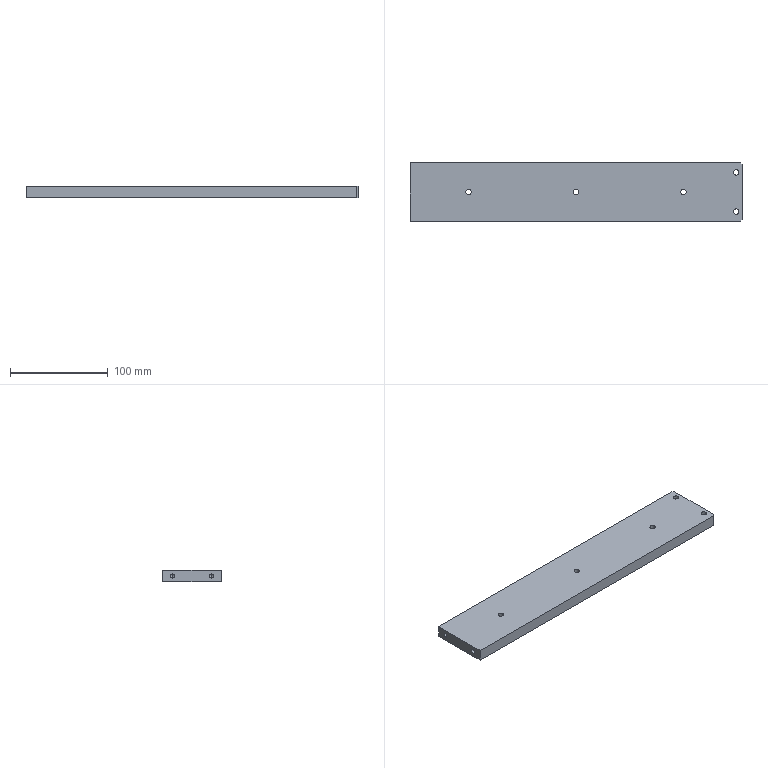Part | SolidWorks | features HoleWzd 3, Chamfer 1, Extrusion 1 | 1 solid | 41 faces | box 340 x 60 x 12 mm | volume 241410 mm3 | cylinder 24 | plane 13 | cone 4 | commonest cylinder face diameters 5.5 x10 10 x10 4.2 x4
STEP:
#1=CARTESIAN_POINT('',(115.,0.,-0.3));
#2=VERTEX_POINT('',#1);
#3=CARTESIAN_POINT('',(105.,0.,-0.3));
#4=VERTEX_POINT('',#3);
#5=CARTESIAN_POINT('',(110.,0.,-0.3));
#6=DIRECTION('',(0.,0.,-1.));
#7=DIRECTION('',(-1.,0.,0.));
#8=AXIS2_PLACEMENT_3D('',#5,#6,#7);
#9=CIRCLE('',#8,5.);
#10=EDGE_CURVE('',#2,#4,#9,.T.);
#11=ORIENTED_EDGE('',*,*,#10,.F.);
#12=CARTESIAN_POINT('',(115.,0.,-6.));
#13=VERTEX_POINT('',#12);
#14=CARTESIAN_POINT('',(115.,0.,-6.));
#15=DIRECTION('',(0.,0.,-1.));
#16=VECTOR('',#15,1000.);
#17=LINE('',#14,#16);
#18=EDGE_CURVE('',#2,#13,#17,.T.);
#19=ORIENTED_EDGE('',*,*,#18,.T.);
#20=CARTESIAN_POINT('',(105.,0.,-6.));
#21=VERTEX_POINT('',#20);
#22=CARTESIAN_POINT('',(110.,0.,-6.));
#23=DIRECTION('',(0.,0.,-1.));
#24=DIRECTION('',(-1.,0.,0.));
#25=AXIS2_PLACEMENT_3D('',#22,#23,#24);
#26=CIRCLE('',#25,5.);
#27=EDGE_CURVE('',#13,#21,#26,.T.);
#28=ORIENTED_EDGE('',*,*,#27,.T.);
#29=CARTESIAN_POINT('',(105.,0.,-6.));
#30=DIRECTION('',(0.,0.,-1.));
#31=VECTOR('',#30,1000.);
#32=LINE('',#29,#31);
#33=EDGE_CURVE('',#4,#21,#32,.T.);
#34=ORIENTED_EDGE('',*,*,#33,.F.);
#35=EDGE_LOOP('',(#11,#19,#28,#34));
#36=FACE_OUTER_BOUND('',#35,.T.);
#37=CARTESIAN_POINT('',(110.,0.,-6.));
#38=DIRECTION('',(0.,0.,-1.));
#39=DIRECTION('',(-1.,0.,0.));
#40=AXIS2_PLACEMENT_3D('',#37,#38,#39);
#41=CYLINDRICAL_SURFACE('',#40,5.);
#42=ADVANCED_FACE('',(#36),#41,.F.);
#43=CARTESIAN_POINT('',(112.75,0.,6.));
#44=VERTEX_POINT('',#43);
#45=CARTESIAN_POINT('',(107.25,0.,6.));
#46=VERTEX_POINT('',#45);
#47=CARTESIAN_POINT('',(110.,0.,6.));
#48=DIRECTION('',(0.,0.,-1.));
#49=DIRECTION('',(-1.,0.,0.));
#50=AXIS2_PLACEMENT_3D('',#47,#48,#49);
#51=CIRCLE('',#50,2.75);
#52=EDGE_CURVE('',#44,#46,#51,.T.);
#53=ORIENTED_EDGE('',*,*,#52,.F.);
#54=CARTESIAN_POINT('',(112.75,0.,-0.3));
#55=VERTEX_POINT('',#54);
#56=CARTESIAN_POINT('',(112.75,0.,-6.));
#57=DIRECTION('',(0.,0.,-1.));
#58=VECTOR('',#57,1000.);
#59=LINE('',#56,#58);
#60=EDGE_CURVE('',#44,#55,#59,.T.);
#61=ORIENTED_EDGE('',*,*,#60,.T.);
#62=CARTESIAN_POINT('',(107.25,0.,-0.3));
#63=VERTEX_POINT('',#62);
#64=CARTESIAN_POINT('',(110.,0.,-0.3));
#65=DIRECTION('',(0.,0.,-1.));
#66=DIRECTION('',(-1.,0.,0.));
#67=AXIS2_PLACEMENT_3D('',#64,#65,#66);
#68=CIRCLE('',#67,2.75);
#69=EDGE_CURVE('',#55,#63,#68,.T.);
#70=ORIENTED_EDGE('',*,*,#69,.T.);
#71=CARTESIAN_POINT('',(107.25,0.,-6.));
#72=DIRECTION('',(0.,0.,-1.));
#73=VECTOR('',#72,1000.);
#74=LINE('',#71,#73);
#75=EDGE_CURVE('',#46,#63,#74,.T.);
#76=ORIENTED_EDGE('',*,*,#75,.F.);
#77=EDGE_LOOP('',(#53,#61,#70,#76));
#78=FACE_OUTER_BOUND('',#77,.T.);
#79=CARTESIAN_POINT('',(110.,0.,-6.));
#80=DIRECTION('',(0.,0.,-1.));
#81=DIRECTION('',(-1.,0.,0.));
#82=AXIS2_PLACEMENT_3D('',#79,#80,#81);
#83=CYLINDRICAL_SURFACE('',#82,2.75);
#84=ADVANCED_FACE('',(#78),#83,.F.);
#85=CARTESIAN_POINT('',(-105.,0.,-0.3));
#86=VERTEX_POINT('',#85);
#87=CARTESIAN_POINT('',(-115.,0.,-0.3));
#88=VERTEX_POINT('',#87);
#89=CARTESIAN_POINT('',(-110.,0.,-0.3));
#90=DIRECTION('',(0.,0.,-1.));
#91=DIRECTION('',(-1.,0.,0.));
#92=AXIS2_PLACEMENT_3D('',#89,#90,#91);
#93=CIRCLE('',#92,5.);
#94=EDGE_CURVE('',#86,#88,#93,.T.);
#95=ORIENTED_EDGE('',*,*,#94,.F.);
#96=CARTESIAN_POINT('',(-105.,0.,-6.));
#97=VERTEX_POINT('',#96);
#98=CARTESIAN_POINT('',(-105.,0.,-6.));
#99=DIRECTION('',(0.,0.,-1.));
#100=VECTOR('',#99,1000.);
#101=LINE('',#98,#100);
#102=EDGE_CURVE('',#86,#97,#101,.T.);
#103=ORIENTED_EDGE('',*,*,#102,.T.);
#104=CARTESIAN_POINT('',(-115.,0.,-6.));
#105=VERTEX_POINT('',#104);
#106=CARTESIAN_POINT('',(-110.,0.,-6.));
#107=DIRECTION('',(0.,0.,-1.));
#108=DIRECTION('',(-1.,0.,0.));
#109=AXIS2_PLACEMENT_3D('',#106,#107,#108);
#110=CIRCLE('',#109,5.);
#111=EDGE_CURVE('',#97,#105,#110,.T.);
#112=ORIENTED_EDGE('',*,*,#111,.T.);
#113=CARTESIAN_POINT('',(-115.,0.,-6.));
#114=DIRECTION('',(0.,0.,-1.));
#115=VECTOR('',#114,1000.);
#116=LINE('',#113,#115);
#117=EDGE_CURVE('',#88,#105,#116,.T.);
#118=ORIENTED_EDGE('',*,*,#117,.F.);
#119=EDGE_LOOP('',(#95,#103,#112,#118));
#120=FACE_OUTER_BOUND('',#119,.T.);
#121=CARTESIAN_POINT('',(-110.,0.,-6.));
#122=DIRECTION('',(0.,0.,-1.));
#123=DIRECTION('',(-1.,0.,0.));
#124=AXIS2_PLACEMENT_3D('',#121,#122,#123);
#125=CYLINDRICAL_SURFACE('',#124,5.);
#126=ADVANCED_FACE('',(#120),#125,.F.);
#127=CARTESIAN_POINT('',(-107.25,0.,6.));
#128=VERTEX_POINT('',#127);
#129=CARTESIAN_POINT('',(-112.75,0.,6.));
#130=VERTEX_POINT('',#129);
#131=CARTESIAN_POINT('',(-110.,0.,6.));
#132=DIRECTION('',(0.,0.,-1.));
#133=DIRECTION('',(-1.,0.,0.));
#134=AXIS2_PLACEMENT_3D('',#131,#132,#133);
#135=CIRCLE('',#134,2.75);
#136=EDGE_CURVE('',#128,#130,#135,.T.);
#137=ORIENTED_EDGE('',*,*,#136,.F.);
#138=CARTESIAN_POINT('',(-107.25,0.,-0.3));
#139=VERTEX_POINT('',#138);
#140=CARTESIAN_POINT('',(-107.25,0.,-6.));
#141=DIRECTION('',(0.,0.,-1.));
#142=VECTOR('',#141,1000.);
#143=LINE('',#140,#142);
#144=EDGE_CURVE('',#128,#139,#143,.T.);
#145=ORIENTED_EDGE('',*,*,#144,.T.);
#146=CARTESIAN_POINT('',(-112.75,0.,-0.3));
#147=VERTEX_POINT('',#146);
#148=CARTESIAN_POINT('',(-110.,0.,-0.3));
#149=DIRECTION('',(0.,0.,-1.));
#150=DIRECTION('',(-1.,0.,0.));
#151=AXIS2_PLACEMENT_3D('',#148,#149,#150);
#152=CIRCLE('',#151,2.75);
#153=EDGE_CURVE('',#139,#147,#152,.T.);
#154=ORIENTED_EDGE('',*,*,#153,.T.);
#155=CARTESIAN_POINT('',(-112.75,0.,-6.));
#156=DIRECTION('',(0.,0.,-1.));
#157=VECTOR('',#156,1000.);
#158=LINE('',#155,#157);
#159=EDGE_CURVE('',#130,#147,#158,.T.);
#160=ORIENTED_EDGE('',*,*,#159,.F.);
#161=EDGE_LOOP('',(#137,#145,#154,#160));
#162=FACE_OUTER_BOUND('',#161,.T.);
#163=CARTESIAN_POINT('',(-110.,0.,-6.));
#164=DIRECTION('',(0.,0.,-1.));
#165=DIRECTION('',(-1.,0.,0.));
#166=AXIS2_PLACEMENT_3D('',#163,#164,#165);
#167=CYLINDRICAL_SURFACE('',#166,2.75);
#168=ADVANCED_FACE('',(#162),#167,.F.);
#169=CARTESIAN_POINT('',(5.,0.,-0.3));
#170=VERTEX_POINT('',#169);
#171=CARTESIAN_POINT('',(-5.,0.,-0.3));
#172=VERTEX_POINT('',#171);
#173=CARTESIAN_POINT('',(0.,0.,-0.3));
#174=DIRECTION('',(0.,0.,-1.));
#175=DIRECTION('',(-1.,0.,0.));
#176=AXIS2_PLACEMENT_3D('',#173,#174,#175);
#177=CIRCLE('',#176,5.);
#178=EDGE_CURVE('',#170,#172,#177,.T.);
#179=ORIENTED_EDGE('',*,*,#178,.F.);
#180=CARTESIAN_POINT('',(5.,0.,-6.));
#181=VERTEX_POINT('',#180);
#182=CARTESIAN_POINT('',(5.,0.,-6.));
#183=DIRECTION('',(0.,0.,-1.));
#184=VECTOR('',#183,1000.);
#185=LINE('',#182,#184);
#186=EDGE_CURVE('',#170,#181,#185,.T.);
#187=ORIENTED_EDGE('',*,*,#186,.T.);
#188=CARTESIAN_POINT('',(-5.,0.,-6.));
#189=VERTEX_POINT('',#188);
#190=CARTESIAN_POINT('',(0.,0.,-6.));
#191=DIRECTION('',(0.,0.,-1.));
#192=DIRECTION('',(-1.,0.,0.));
#193=AXIS2_PLACEMENT_3D('',#190,#191,#192);
#194=CIRCLE('',#193,5.);
#195=EDGE_CURVE('',#181,#189,#194,.T.);
#196=ORIENTED_EDGE('',*,*,#195,.T.);
#197=CARTESIAN_POINT('',(-5.,0.,-6.));
#198=DIRECTION('',(0.,0.,-1.));
#199=VECTOR('',#198,1000.);
#200=LINE('',#197,#199);
#201=EDGE_CURVE('',#172,#189,#200,.T.);
#202=ORIENTED_EDGE('',*,*,#201,.F.);
#203=EDGE_LOOP('',(#179,#187,#196,#202));
#204=FACE_OUTER_BOUND('',#203,.T.);
#205=CARTESIAN_POINT('',(0.,0.,-6.));
#206=DIRECTION('',(0.,0.,-1.));
#207=DIRECTION('',(-1.,0.,0.));
#208=AXIS2_PLACEMENT_3D('',#205,#206,#207);
#209=CYLINDRICAL_SURFACE('',#208,5.);
#210=ADVANCED_FACE('',(#204),#209,.F.);
#211=CARTESIAN_POINT('',(2.75,0.,6.));
#212=VERTEX_POINT('',#211);
#213=CARTESIAN_POINT('',(-2.75,0.,6.));
#214=VERTEX_POINT('',#213);
#215=CARTESIAN_POINT('',(0.,0.,6.));
#216=DIRECTION('',(0.,0.,-1.));
#217=DIRECTION('',(-1.,0.,0.));
#218=AXIS2_PLACEMENT_3D('',#215,#216,#217);
#219=CIRCLE('',#218,2.75);
#220=EDGE_CURVE('',#212,#214,#219,.T.);
#221=ORIENTED_EDGE('',*,*,#220,.F.);
#222=CARTESIAN_POINT('',(2.75,0.,-0.3));
#223=VERTEX_POINT('',#222);
#224=CARTESIAN_POINT('',(2.75,0.,-6.));
#225=DIRECTION('',(0.,0.,-1.));
#226=VECTOR('',#225,1000.);
#227=LINE('',#224,#226);
#228=EDGE_CURVE('',#212,#223,#227,.T.);
#229=ORIENTED_EDGE('',*,*,#228,.T.);
#230=CARTESIAN_POINT('',(-2.75,0.,-0.3));
#231=VERTEX_POINT('',#230);
#232=CARTESIAN_POINT('',(0.,0.,-0.3));
#233=DIRECTION('',(0.,0.,-1.));
#234=DIRECTION('',(-1.,0.,0.));
#235=AXIS2_PLACEMENT_3D('',#232,#233,#234);
#236=CIRCLE('',#235,2.75);
#237=EDGE_CURVE('',#223,#231,#236,.T.);
#238=ORIENTED_EDGE('',*,*,#237,.T.);
#239=CARTESIAN_POINT('',(-2.75,0.,-6.));
#240=DIRECTION('',(0.,0.,-1.));
#241=VECTOR('',#240,1000.);
#242=LINE('',#239,#241);
#243=EDGE_CURVE('',#214,#231,#242,.T.);
#244=ORIENTED_EDGE('',*,*,#243,.F.);
#245=EDGE_LOOP('',(#221,#229,#238,#244));
#246=FACE_OUTER_BOUND('',#245,.T.);
#247=CARTESIAN_POINT('',(0.,0.,-6.));
#248=DIRECTION('',(0.,0.,-1.));
#249=DIRECTION('',(-1.,0.,0.));
#250=AXIS2_PLACEMENT_3D('',#247,#248,#249);
#251=CYLINDRICAL_SURFACE('',#250,2.75);
#252=ADVANCED_FACE('',(#246),#251,.F.);
#253=CARTESIAN_POINT('',(169.,20.,-0.3));
#254=VERTEX_POINT('',#253);
#255=CARTESIAN_POINT('',(159.,20.,-0.3));
#256=VERTEX_POINT('',#255);
#257=CARTESIAN_POINT('',(164.,20.,-0.3));
#258=DIRECTION('',(0.,0.,-1.));
#259=DIRECTION('',(-1.,0.,0.));
#260=AXIS2_PLACEMENT_3D('',#257,#258,#259);
#261=CIRCLE('',#260,5.);
#262=EDGE_CURVE('',#254,#256,#261,.T.);
#263=ORIENTED_EDGE('',*,*,#262,.F.);
#264=CARTESIAN_POINT('',(169.,20.,-6.));
#265=VERTEX_POINT('',#264);
#266=CARTESIAN_POINT('',(169.,20.,-6.));
#267=DIRECTION('',(0.,0.,-1.));
#268=VECTOR('',#267,1000.);
#269=LINE('',#266,#268);
#270=EDGE_CURVE('',#254,#265,#269,.T.);
#271=ORIENTED_EDGE('',*,*,#270,.T.);
#272=CARTESIAN_POINT('',(159.,20.,-6.));
#273=VERTEX_POINT('',#272);
#274=CARTESIAN_POINT('',(164.,20.,-6.));
#275=DIRECTION('',(0.,0.,-1.));
#276=DIRECTION('',(-1.,0.,0.));
#277=AXIS2_PLACEMENT_3D('',#274,#275,#276);
#278=CIRCLE('',#277,5.);
#279=EDGE_CURVE('',#265,#273,#278,.T.);
#280=ORIENTED_EDGE('',*,*,#279,.T.);
#281=CARTESIAN_POINT('',(159.,20.,-6.));
#282=DIRECTION('',(0.,0.,-1.));
#283=VECTOR('',#282,1000.);
#284=LINE('',#281,#283);
#285=EDGE_CURVE('',#256,#273,#284,.T.);
#286=ORIENTED_EDGE('',*,*,#285,.F.);
#287=EDGE_LOOP('',(#263,#271,#280,#286));
#288=FACE_OUTER_BOUND('',#287,.T.);
#289=CARTESIAN_POINT('',(164.,20.,-6.));
#290=DIRECTION('',(0.,0.,-1.));
#291=DIRECTION('',(-1.,0.,0.));
#292=AXIS2_PLACEMENT_3D('',#289,#290,#291);
#293=CYLINDRICAL_SURFACE('',#292,5.);
#294=ADVANCED_FACE('',(#288),#293,.F.);
#295=CARTESIAN_POINT('',(166.75,20.,6.));
#296=VERTEX_POINT('',#295);
#297=CARTESIAN_POINT('',(161.25,20.,6.));
#298=VERTEX_POINT('',#297);
#299=CARTESIAN_POINT('',(164.,20.,6.));
#300=DIRECTION('',(0.,0.,-1.));
#301=DIRECTION('',(-1.,0.,0.));
#302=AXIS2_PLACEMENT_3D('',#299,#300,#301);
#303=CIRCLE('',#302,2.75);
#304=EDGE_CURVE('',#296,#298,#303,.T.);
#305=ORIENTED_EDGE('',*,*,#304,.F.);
#306=CARTESIAN_POINT('',(166.75,20.,-0.3));
#307=VERTEX_POINT('',#306);
#308=CARTESIAN_POINT('',(166.75,20.,-6.));
#309=DIRECTION('',(0.,0.,-1.));
#310=VECTOR('',#309,1000.);
#311=LINE('',#308,#310);
#312=EDGE_CURVE('',#296,#307,#311,.T.);
#313=ORIENTED_EDGE('',*,*,#312,.T.);
#314=CARTESIAN_POINT('',(161.25,20.,-0.3));
#315=VERTEX_POINT('',#314);
#316=CARTESIAN_POINT('',(164.,20.,-0.3));
#317=DIRECTION('',(0.,0.,-1.));
#318=DIRECTION('',(-1.,0.,0.));
#319=AXIS2_PLACEMENT_3D('',#316,#317,#318);
#320=CIRCLE('',#319,2.75);
#321=EDGE_CURVE('',#307,#315,#320,.T.);
#322=ORIENTED_EDGE('',*,*,#321,.T.);
#323=CARTESIAN_POINT('',(161.25,20.,-6.));
#324=DIRECTION('',(0.,0.,-1.));
#325=VECTOR('',#324,1000.);
#326=LINE('',#323,#325);
#327=EDGE_CURVE('',#298,#315,#326,.T.);
#328=ORIENTED_EDGE('',*,*,#327,.F.);
#329=EDGE_LOOP('',(#305,#313,#322,#328));
#330=FACE_OUTER_BOUND('',#329,.T.);
#331=CARTESIAN_POINT('',(164.,20.,-6.));
#332=DIRECTION('',(0.,0.,-1.));
#333=DIRECTION('',(-1.,0.,0.));
#334=AXIS2_PLACEMENT_3D('',#331,#332,#333);
#335=CYLINDRICAL_SURFACE('',#334,2.75);
#336=ADVANCED_FACE('',(#330),#335,.F.);
#337=CARTESIAN_POINT('',(169.,-20.,-0.3));
#338=VERTEX_POINT('',#337);
#339=CARTESIAN_POINT('',(159.,-20.,-0.3));
#340=VERTEX_POINT('',#339);
#341=CARTESIAN_POINT('',(164.,-20.,-0.3));
#342=DIRECTION('',(0.,0.,-1.));
#343=DIRECTION('',(-1.,0.,0.));
#344=AXIS2_PLACEMENT_3D('',#341,#342,#343);
#345=CIRCLE('',#344,5.);
#346=EDGE_CURVE('',#338,#340,#345,.T.);
#347=ORIENTED_EDGE('',*,*,#346,.F.);
#348=CARTESIAN_POINT('',(169.,-20.,-6.));
#349=VERTEX_POINT('',#348);
#350=CARTESIAN_POINT('',(169.,-20.,-6.));
#351=DIRECTION('',(0.,0.,-1.));
#352=VECTOR('',#351,1000.);
#353=LINE('',#350,#352);
#354=EDGE_CURVE('',#338,#349,#353,.T.);
#355=ORIENTED_EDGE('',*,*,#354,.T.);
#356=CARTESIAN_POINT('',(159.,-20.,-6.));
#357=VERTEX_POINT('',#356);
#358=CARTESIAN_POINT('',(164.,-20.,-6.));
#359=DIRECTION('',(0.,0.,-1.));
#360=DIRECTION('',(-1.,0.,0.));
#361=AXIS2_PLACEMENT_3D('',#358,#359,#360);
#362=CIRCLE('',#361,5.);
#363=EDGE_CURVE('',#349,#357,#362,.T.);
#364=ORIENTED_EDGE('',*,*,#363,.T.);
#365=CARTESIAN_POINT('',(159.,-20.,-6.));
#366=DIRECTION('',(0.,0.,-1.));
#367=VECTOR('',#366,1000.);
#368=LINE('',#365,#367);
#369=EDGE_CURVE('',#340,#357,#368,.T.);
#370=ORIENTED_EDGE('',*,*,#369,.F.);
#371=EDGE_LOOP('',(#347,#355,#364,#370));
#372=FACE_OUTER_BOUND('',#371,.T.);
#373=CARTESIAN_POINT('',(164.,-20.,-6.));
#374=DIRECTION('',(0.,0.,-1.));
#375=DIRECTION('',(-1.,0.,0.));
#376=AXIS2_PLACEMENT_3D('',#373,#374,#375);
#377=CYLINDRICAL_SURFACE('',#376,5.);
#378=ADVANCED_FACE('',(#372),#377,.F.);
#379=CARTESIAN_POINT('',(166.75,-20.,6.));
#380=VERTEX_POINT('',#379);
#381=CARTESIAN_POINT('',(161.25,-20.,6.));
#382=VERTEX_POINT('',#381);
#383=CARTESIAN_POINT('',(164.,-20.,6.));
#384=DIRECTION('',(0.,0.,-1.));
#385=DIRECTION('',(-1.,0.,0.));
#386=AXIS2_PLACEMENT_3D('',#383,#384,#385);
#387=CIRCLE('',#386,2.75);
#388=EDGE_CURVE('',#380,#382,#387,.T.);
#389=ORIENTED_EDGE('',*,*,#388,.F.);
#390=CARTESIAN_POINT('',(166.75,-20.,-0.3));
#391=VERTEX_POINT('',#390);
#392=CARTESIAN_POINT('',(166.75,-20.,-6.));
#393=DIRECTION('',(0.,0.,-1.));
#394=VECTOR('',#393,1000.);
#395=LINE('',#392,#394);
#396=EDGE_CURVE('',#380,#391,#395,.T.);
#397=ORIENTED_EDGE('',*,*,#396,.T.);
#398=CARTESIAN_POINT('',(161.25,-20.,-0.3));
#399=VERTEX_POINT('',#398);
#400=CARTESIAN_POINT('',(164.,-20.,-0.3));
#401=DIRECTION('',(0.,0.,-1.));
#402=DIRECTION('',(-1.,0.,0.));
#403=AXIS2_PLACEMENT_3D('',#400,#401,#402);
#404=CIRCLE('',#403,2.75);
#405=EDGE_CURVE('',#391,#399,#404,.T.);
#406=ORIENTED_EDGE('',*,*,#405,.T.);
#407=CARTESIAN_POINT('',(161.25,-20.,-6.));
#408=DIRECTION('',(0.,0.,-1.));
#409=VECTOR('',#408,1000.);
#410=LINE('',#407,#409);
#411=EDGE_CURVE('',#382,#399,#410,.T.);
#412=ORIENTED_EDGE('',*,*,#411,.F.);
#413=EDGE_LOOP('',(#389,#397,#406,#412));
#414=FACE_OUTER_BOUND('',#413,.T.);
#415=CARTESIAN_POINT('',(164.,-20.,-6.));
#416=DIRECTION('',(0.,0.,-1.));
#417=DIRECTION('',(-1.,0.,0.));
#418=AXIS2_PLACEMENT_3D('',#415,#416,#417);
#419=CYLINDRICAL_SURFACE('',#418,2.75);
#420=ADVANCED_FACE('',(#414),#419,.F.);
#421=CARTESIAN_POINT('',(-157.6,20.,-2.1));
#422=VERTEX_POINT('',#421);
#423=CARTESIAN_POINT('',(-157.6,20.,2.1));
#424=VERTEX_POINT('',#423);
#425=CARTESIAN_POINT('',(-157.6,20.,0.));
#426=DIRECTION('',(-1.,0.,0.));
#427=DIRECTION('',(0.,0.,1.));
#428=AXIS2_PLACEMENT_3D('',#425,#426,#427);
#429=CIRCLE('',#428,2.1);
#430=EDGE_CURVE('',#422,#424,#429,.T.);
#431=ORIENTED_EDGE('',*,*,#430,.F.);
#432=CARTESIAN_POINT('',(-170.,20.,-2.1));
#433=VERTEX_POINT('',#432);
#434=CARTESIAN_POINT('',(-170.,20.,-2.1));
#435=DIRECTION('',(-1.,0.,0.));
#436=VECTOR('',#435,1000.);
#437=LINE('',#434,#436);
#438=EDGE_CURVE('',#422,#433,#437,.T.);
#439=ORIENTED_EDGE('',*,*,#438,.T.);
#440=CARTESIAN_POINT('',(-170.,20.,2.1));
#441=VERTEX_POINT('',#440);
#442=CARTESIAN_POINT('',(-170.,20.,0.));
#443=DIRECTION('',(-1.,0.,0.));
#444=DIRECTION('',(0.,0.,1.));
#445=AXIS2_PLACEMENT_3D('',#442,#443,#444);
#446=CIRCLE('',#445,2.1);
#447=EDGE_CURVE('',#433,#441,#446,.T.);
#448=ORIENTED_EDGE('',*,*,#447,.T.);
#449=CARTESIAN_POINT('',(-170.,20.,2.1));
#450=DIRECTION('',(-1.,0.,0.));
#451=VECTOR('',#450,1000.);
#452=LINE('',#449,#451);
#453=EDGE_CURVE('',#424,#441,#452,.T.);
#454=ORIENTED_EDGE('',*,*,#453,.F.);
#455=EDGE_LOOP('',(#431,#439,#448,#454));
#456=FACE_OUTER_BOUND('',#455,.T.);
#457=CARTESIAN_POINT('',(-170.,20.,0.));
#458=DIRECTION('',(-1.,0.,0.));
#459=DIRECTION('',(0.,0.,1.));
#460=AXIS2_PLACEMENT_3D('',#457,#458,#459);
#461=CYLINDRICAL_SURFACE('',#460,2.1);
#462=ADVANCED_FACE('',(#456),#461,.F.);
#463=CARTESIAN_POINT('',(-156.338,20.,0.));
#464=VERTEX_POINT('',#463);
#465=CARTESIAN_POINT('',(-157.6,20.,2.1));
#466=DIRECTION('',(-0.515,0.,0.8572));
#467=VECTOR('',#466,1000.);
#468=LINE('',#465,#467);
#469=EDGE_CURVE('',#464,#424,#468,.T.);
#470=ORIENTED_EDGE('',*,*,#469,.F.);
#471=CARTESIAN_POINT('',(-157.6,20.,-2.1));
#472=DIRECTION('',(-0.515,0.,-0.8572));
#473=VECTOR('',#472,1000.);
#474=LINE('',#471,#473);
#475=EDGE_CURVE('',#464,#422,#474,.T.);
#476=ORIENTED_EDGE('',*,*,#475,.T.);
#477=ORIENTED_EDGE('',*,*,#430,.T.);
#478=EDGE_LOOP('',(#470,#476,#477));
#479=FACE_OUTER_BOUND('',#478,.T.);
#480=CARTESIAN_POINT('',(-157.6,20.,0.));
#481=DIRECTION('',(-1.,0.,0.));
#482=DIRECTION('',(0.,0.,1.));
#483=AXIS2_PLACEMENT_3D('',#480,#481,#482);
#484=CONICAL_SURFACE('',#483,2.1,1.03);
#485=ADVANCED_FACE('',(#479),#484,.F.);
#486=CARTESIAN_POINT('',(-157.6,-20.,-2.1));
#487=VERTEX_POINT('',#486);
#488=CARTESIAN_POINT('',(-157.6,-20.,2.1));
#489=VERTEX_POINT('',#488);
#490=CARTESIAN_POINT('',(-157.6,-20.,0.));
#491=DIRECTION('',(-1.,0.,0.));
#492=DIRECTION('',(0.,0.,1.));
#493=AXIS2_PLACEMENT_3D('',#490,#491,#492);
#494=CIRCLE('',#493,2.1);
#495=EDGE_CURVE('',#487,#489,#494,.T.);
#496=ORIENTED_EDGE('',*,*,#495,.F.);
#497=CARTESIAN_POINT('',(-170.,-20.,-2.1));
#498=VERTEX_POINT('',#497);
#499=CARTESIAN_POINT('',(-170.,-20.,-2.1));
#500=DIRECTION('',(-1.,0.,0.));
#501=VECTOR('',#500,1000.);
#502=LINE('',#499,#501);
#503=EDGE_CURVE('',#487,#498,#502,.T.);
#504=ORIENTED_EDGE('',*,*,#503,.T.);
#505=CARTESIAN_POINT('',(-170.,-20.,2.1));
#506=VERTEX_POINT('',#505);
#507=CARTESIAN_POINT('',(-170.,-20.,0.));
#508=DIRECTION('',(-1.,0.,0.));
#509=DIRECTION('',(0.,0.,1.));
#510=AXIS2_PLACEMENT_3D('',#507,#508,#509);
#511=CIRCLE('',#510,2.1);
#512=EDGE_CURVE('',#498,#506,#511,.T.);
#513=ORIENTED_EDGE('',*,*,#512,.T.);
#514=CARTESIAN_POINT('',(-170.,-20.,2.1));
#515=DIRECTION('',(-1.,0.,0.));
#516=VECTOR('',#515,1000.);
#517=LINE('',#514,#516);
#518=EDGE_CURVE('',#489,#506,#517,.T.);
#519=ORIENTED_EDGE('',*,*,#518,.F.);
#520=EDGE_LOOP('',(#496,#504,#513,#519));
#521=FACE_OUTER_BOUND('',#520,.T.);
#522=CARTESIAN_POINT('',(-170.,-20.,0.));
#523=DIRECTION('',(-1.,0.,0.));
#524=DIRECTION('',(0.,0.,1.));
#525=AXIS2_PLACEMENT_3D('',#522,#523,#524);
#526=CYLINDRICAL_SURFACE('',#525,2.1);
#527=ADVANCED_FACE('',(#521),#526,.F.);
#528=CARTESIAN_POINT('',(-156.338,-20.,0.));
#529=VERTEX_POINT('',#528);
#530=CARTESIAN_POINT('',(-157.6,-20.,2.1));
#531=DIRECTION('',(-0.515,0.,0.8572));
#532=VECTOR('',#531,1000.);
#533=LINE('',#530,#532);
#534=EDGE_CURVE('',#529,#489,#533,.T.);
#535=ORIENTED_EDGE('',*,*,#534,.F.);
#536=CARTESIAN_POINT('',(-157.6,-20.,-2.1));
#537=DIRECTION('',(-0.515,0.,-0.8572));
#538=VECTOR('',#537,1000.);
#539=LINE('',#536,#538);
#540=EDGE_CURVE('',#529,#487,#539,.T.);
#541=ORIENTED_EDGE('',*,*,#540,.T.);
#542=ORIENTED_EDGE('',*,*,#495,.T.);
#543=EDGE_LOOP('',(#535,#541,#542));
#544=FACE_OUTER_BOUND('',#543,.T.);
#545=CARTESIAN_POINT('',(-157.6,-20.,0.));
#546=DIRECTION('',(-1.,0.,0.));
#547=DIRECTION('',(0.,0.,1.));
#548=AXIS2_PLACEMENT_3D('',#545,#546,#547);
#549=CONICAL_SURFACE('',#548,2.1,1.03);
#550=ADVANCED_FACE('',(#544),#549,.F.);
#551=CARTESIAN_POINT('',(170.,-28.,6.));
#552=VERTEX_POINT('',#551);
#553=CARTESIAN_POINT('',(170.,28.,6.));
#554=VERTEX_POINT('',#553);
#555=CARTESIAN_POINT('',(170.,-30.,6.));
#556=DIRECTION('',(0.,1.,0.));
#557=VECTOR('',#556,1000.);
#558=LINE('',#555,#557);
#559=EDGE_CURVE('',#552,#554,#558,.T.);
#560=ORIENTED_EDGE('',*,*,#559,.F.);
#561=CARTESIAN_POINT('',(170.,-28.,-6.));
#562=VERTEX_POINT('',#561);
#563=CARTESIAN_POINT('',(170.,-28.,6.));
#564=DIRECTION('',(0.,0.,-1.));
#565=VECTOR('',#564,1000.);
#566=LINE('',#563,#565);
#567=EDGE_CURVE('',#552,#562,#566,.T.);
#568=ORIENTED_EDGE('',*,*,#567,.T.);
#569=CARTESIAN_POINT('',(170.,28.,-6.));
#570=VERTEX_POINT('',#569);
#571=CARTESIAN_POINT('',(170.,-30.,-6.));
#572=DIRECTION('',(0.,1.,0.));
#573=VECTOR('',#572,1000.);
#574=LINE('',#571,#573);
#575=EDGE_CURVE('',#562,#570,#574,.T.);
#576=ORIENTED_EDGE('',*,*,#575,.T.);
#577=CARTESIAN_POINT('',(170.,28.,6.));
#578=DIRECTION('',(0.,0.,1.));
#579=VECTOR('',#578,1000.);
#580=LINE('',#577,#579);
#581=EDGE_CURVE('',#570,#554,#580,.T.);
#582=ORIENTED_EDGE('',*,*,#581,.T.);
#583=EDGE_LOOP('',(#560,#568,#576,#582));
#584=FACE_OUTER_BOUND('',#583,.T.);
#585=CARTESIAN_POINT('',(170.,-30.,6.));
#586=DIRECTION('',(-1.,0.,0.));
#587=DIRECTION('',(0.,0.,1.));
#588=AXIS2_PLACEMENT_3D('',#585,#586,#587);
#589=PLANE('',#588);
#590=ADVANCED_FACE('',(#584),#589,.F.);
#591=CARTESIAN_POINT('',(168.,30.,6.));
#592=VERTEX_POINT('',#591);
#593=CARTESIAN_POINT('',(-170.,30.,6.));
#594=VERTEX_POINT('',#593);
#595=CARTESIAN_POINT('',(-170.,30.,6.));
#596=DIRECTION('',(-1.,0.,0.));
#597=VECTOR('',#596,1000.);
#598=LINE('',#595,#597);
#599=EDGE_CURVE('',#592,#594,#598,.T.);
#600=ORIENTED_EDGE('',*,*,#599,.F.);
#601=CARTESIAN_POINT('',(168.,30.,-6.));
#602=VERTEX_POINT('',#601);
#603=CARTESIAN_POINT('',(168.,30.,6.));
#604=DIRECTION('',(0.,0.,-1.));
#605=VECTOR('',#604,1000.);
#606=LINE('',#603,#605);
#607=EDGE_CURVE('',#592,#602,#606,.T.);
#608=ORIENTED_EDGE('',*,*,#607,.T.);
#609=CARTESIAN_POINT('',(-170.,30.,-6.));
#610=VERTEX_POINT('',#609);
#611=CARTESIAN_POINT('',(-170.,30.,-6.));
#612=DIRECTION('',(-1.,0.,0.));
#613=VECTOR('',#612,1000.);
#614=LINE('',#611,#613);
#615=EDGE_CURVE('',#602,#610,#614,.T.);
#616=ORIENTED_EDGE('',*,*,#615,.T.);
#617=CARTESIAN_POINT('',(-170.,30.,6.));
#618=DIRECTION('',(0.,0.,-1.));
#619=VECTOR('',#618,1000.);
#620=LINE('',#617,#619);
#621=EDGE_CURVE('',#594,#610,#620,.T.);
#622=ORIENTED_EDGE('',*,*,#621,.F.);
#623=EDGE_LOOP('',(#600,#608,#616,#622));
#624=FACE_OUTER_BOUND('',#623,.T.);
#625=CARTESIAN_POINT('',(-170.,30.,6.));
#626=DIRECTION('',(0.,-1.,0.));
#627=DIRECTION('',(0.,0.,-1.));
#628=AXIS2_PLACEMENT_3D('',#625,#626,#627);
#629=PLANE('',#628);
#630=ADVANCED_FACE('',(#624),#629,.F.);
#631=CARTESIAN_POINT('',(-170.,20.,0.));
#632=DIRECTION('',(-1.,0.,0.));
#633=DIRECTION('',(0.,0.,1.));
#634=AXIS2_PLACEMENT_3D('',#631,#632,#633);
#635=CIRCLE('',#634,2.1);
#636=EDGE_CURVE('',#441,#433,#635,.T.);
#637=ORIENTED_EDGE('',*,*,#636,.F.);
#638=ORIENTED_EDGE('',*,*,#447,.F.);
#639=EDGE_LOOP('',(#637,#638));
#640=FACE_BOUND('',#639,.T.);
#641=CARTESIAN_POINT('',(-170.,-20.,0.));
#642=DIRECTION('',(-1.,0.,0.));
#643=DIRECTION('',(0.,0.,1.));
#644=AXIS2_PLACEMENT_3D('',#641,#642,#643);
#645=CIRCLE('',#644,2.1);
#646=EDGE_CURVE('',#506,#498,#645,.T.);
#647=ORIENTED_EDGE('',*,*,#646,.F.);
#648=ORIENTED_EDGE('',*,*,#512,.F.);
#649=EDGE_LOOP('',(#647,#648));
#650=FACE_BOUND('',#649,.T.);
#651=CARTESIAN_POINT('',(-170.,-30.,-6.));
#652=VERTEX_POINT('',#651);
#653=CARTESIAN_POINT('',(-170.,-30.,-6.));
#654=DIRECTION('',(0.,-1.,0.));
#655=VECTOR('',#654,1000.);
#656=LINE('',#653,#655);
#657=EDGE_CURVE('',#610,#652,#656,.T.);
#658=ORIENTED_EDGE('',*,*,#657,.T.);
#659=CARTESIAN_POINT('',(-170.,-30.,6.));
#660=VERTEX_POINT('',#659);
#661=CARTESIAN_POINT('',(-170.,-30.,6.));
#662=DIRECTION('',(0.,0.,-1.));
#663=VECTOR('',#662,1000.);
#664=LINE('',#661,#663);
#665=EDGE_CURVE('',#660,#652,#664,.T.);
#666=ORIENTED_EDGE('',*,*,#665,.F.);
#667=CARTESIAN_POINT('',(-170.,-30.,6.));
#668=DIRECTION('',(0.,-1.,0.));
#669=VECTOR('',#668,1000.);
#670=LINE('',#667,#669);
#671=EDGE_CURVE('',#594,#660,#670,.T.);
#672=ORIENTED_EDGE('',*,*,#671,.F.);
#673=ORIENTED_EDGE('',*,*,#621,.T.);
#674=EDGE_LOOP('',(#658,#666,#672,#673));
#675=FACE_OUTER_BOUND('',#674,.T.);
#676=CARTESIAN_POINT('',(-170.,-30.,6.));
#677=DIRECTION('',(1.,0.,0.));
#678=DIRECTION('',(0.,0.,-1.));
#679=AXIS2_PLACEMENT_3D('',#676,#677,#678);
#680=PLANE('',#679);
#681=ADVANCED_FACE('',(#640,#650,#675),#680,.F.);
#682=CARTESIAN_POINT('',(168.,-30.,-6.));
#683=VERTEX_POINT('',#682);
#684=CARTESIAN_POINT('',(-170.,-30.,-6.));
#685=DIRECTION('',(1.,0.,0.));
#686=VECTOR('',#685,1000.);
#687=LINE('',#684,#686);
#688=EDGE_CURVE('',#652,#683,#687,.T.);
#689=ORIENTED_EDGE('',*,*,#688,.T.);
#690=CARTESIAN_POINT('',(168.,-30.,6.));
#691=VERTEX_POINT('',#690);
#692=CARTESIAN_POINT('',(168.,-30.,6.));
#693=DIRECTION('',(0.,0.,1.));
#694=VECTOR('',#693,1000.);
#695=LINE('',#692,#694);
#696=EDGE_CURVE('',#683,#691,#695,.T.);
#697=ORIENTED_EDGE('',*,*,#696,.T.);
#698=CARTESIAN_POINT('',(-170.,-30.,6.));
#699=DIRECTION('',(1.,0.,0.));
#700=VECTOR('',#699,1000.);
#701=LINE('',#698,#700);
#702=EDGE_CURVE('',#660,#691,#701,.T.);
#703=ORIENTED_EDGE('',*,*,#702,.F.);
#704=ORIENTED_EDGE('',*,*,#665,.T.);
#705=EDGE_LOOP('',(#689,#697,#703,#704));
#706=FACE_OUTER_BOUND('',#705,.T.);
#707=CARTESIAN_POINT('',(-170.,-30.,6.));
#708=DIRECTION('',(0.,1.,0.));
#709=DIRECTION('',(0.,0.,1.));
#710=AXIS2_PLACEMENT_3D('',#707,#708,#709);
#711=PLANE('',#710);
#712=ADVANCED_FACE('',(#706),#711,.F.);
#713=CARTESIAN_POINT('',(110.,0.,6.));
#714=DIRECTION('',(0.,0.,-1.));
#715=DIRECTION('',(-1.,0.,0.));
#716=AXIS2_PLACEMENT_3D('',#713,#714,#715);
#717=CIRCLE('',#716,2.75);
#718=EDGE_CURVE('',#46,#44,#717,.T.);
#719=ORIENTED_EDGE('',*,*,#718,.T.);
#720=ORIENTED_EDGE('',*,*,#52,.T.);
#721=EDGE_LOOP('',(#719,#720));
#722=FACE_BOUND('',#721,.T.);
#723=CARTESIAN_POINT('',(-110.,0.,6.));
#724=DIRECTION('',(0.,0.,-1.));
#725=DIRECTION('',(-1.,0.,0.));
#726=AXIS2_PLACEMENT_3D('',#723,#724,#725);
#727=CIRCLE('',#726,2.75);
#728=EDGE_CURVE('',#130,#128,#727,.T.);
#729=ORIENTED_EDGE('',*,*,#728,.T.);
#730=ORIENTED_EDGE('',*,*,#136,.T.);
#731=EDGE_LOOP('',(#729,#730));
#732=FACE_BOUND('',#731,.T.);
#733=CARTESIAN_POINT('',(0.,0.,6.));
#734=DIRECTION('',(0.,0.,-1.));
#735=DIRECTION('',(-1.,0.,0.));
#736=AXIS2_PLACEMENT_3D('',#733,#734,#735);
#737=CIRCLE('',#736,2.75);
#738=EDGE_CURVE('',#214,#212,#737,.T.);
#739=ORIENTED_EDGE('',*,*,#738,.T.);
#740=ORIENTED_EDGE('',*,*,#220,.T.);
#741=EDGE_LOOP('',(#739,#740));
#742=FACE_BOUND('',#741,.T.);
#743=CARTESIAN_POINT('',(164.,20.,6.));
#744=DIRECTION('',(0.,0.,-1.));
#745=DIRECTION('',(-1.,0.,0.));
#746=AXIS2_PLACEMENT_3D('',#743,#744,#745);
#747=CIRCLE('',#746,2.75);
#748=EDGE_CURVE('',#298,#296,#747,.T.);
#749=ORIENTED_EDGE('',*,*,#748,.T.);
#750=ORIENTED_EDGE('',*,*,#304,.T.);
#751=EDGE_LOOP('',(#749,#750));
#752=FACE_BOUND('',#751,.T.);
#753=CARTESIAN_POINT('',(164.,-20.,6.));
#754=DIRECTION('',(0.,0.,-1.));
#755=DIRECTION('',(-1.,0.,0.));
#756=AXIS2_PLACEMENT_3D('',#753,#754,#755);
#757=CIRCLE('',#756,2.75);
#758=EDGE_CURVE('',#382,#380,#757,.T.);
#759=ORIENTED_EDGE('',*,*,#758,.T.);
#760=ORIENTED_EDGE('',*,*,#388,.T.);
#761=EDGE_LOOP('',(#759,#760));
#762=FACE_BOUND('',#761,.T.);
#763=ORIENTED_EDGE('',*,*,#702,.T.);
#764=CARTESIAN_POINT('',(170.,-28.,6.));
#765=DIRECTION('',(0.7071,0.7071,0.));
#766=VECTOR('',#765,1000.);
#767=LINE('',#764,#766);
#768=EDGE_CURVE('',#691,#552,#767,.T.);
#769=ORIENTED_EDGE('',*,*,#768,.T.);
#770=ORIENTED_EDGE('',*,*,#559,.T.);
#771=CARTESIAN_POINT('',(168.,30.,6.));
#772=DIRECTION('',(-0.7071,0.7071,0.));
#773=VECTOR('',#772,1000.);
#774=LINE('',#771,#773);
#775=EDGE_CURVE('',#554,#592,#774,.T.);
#776=ORIENTED_EDGE('',*,*,#775,.T.);
#777=ORIENTED_EDGE('',*,*,#599,.T.);
#778=ORIENTED_EDGE('',*,*,#671,.T.);
#779=EDGE_LOOP('',(#763,#769,#770,#776,#777,#778));
#780=FACE_OUTER_BOUND('',#779,.T.);
#781=CARTESIAN_POINT('',(0.,0.,6.));
#782=DIRECTION('',(0.,0.,-1.));
#783=DIRECTION('',(-1.,0.,0.));
#784=AXIS2_PLACEMENT_3D('',#781,#782,#783);
#785=PLANE('',#784);
#786=ADVANCED_FACE('',(#722,#732,#742,#752,#762,#780),#785,.F.);
#787=CARTESIAN_POINT('',(110.,0.,-6.));
#788=DIRECTION('',(0.,0.,-1.));
#789=DIRECTION('',(-1.,0.,0.));
#790=AXIS2_PLACEMENT_3D('',#787,#788,#789);
#791=CIRCLE('',#790,5.);
#792=EDGE_CURVE('',#21,#13,#791,.T.);
#793=ORIENTED_EDGE('',*,*,#792,.F.);
#794=ORIENTED_EDGE('',*,*,#27,.F.);
#795=EDGE_LOOP('',(#793,#794));
#796=FACE_BOUND('',#795,.T.);
#797=CARTESIAN_POINT('',(-110.,0.,-6.));
#798=DIRECTION('',(0.,0.,-1.));
#799=DIRECTION('',(-1.,0.,0.));
#800=AXIS2_PLACEMENT_3D('',#797,#798,#799);
#801=CIRCLE('',#800,5.);
#802=EDGE_CURVE('',#105,#97,#801,.T.);
#803=ORIENTED_EDGE('',*,*,#802,.F.);
#804=ORIENTED_EDGE('',*,*,#111,.F.);
#805=EDGE_LOOP('',(#803,#804));
#806=FACE_BOUND('',#805,.T.);
#807=CARTESIAN_POINT('',(0.,0.,-6.));
#808=DIRECTION('',(0.,0.,-1.));
#809=DIRECTION('',(-1.,0.,0.));
#810=AXIS2_PLACEMENT_3D('',#807,#808,#809);
#811=CIRCLE('',#810,5.);
#812=EDGE_CURVE('',#189,#181,#811,.T.);
#813=ORIENTED_EDGE('',*,*,#812,.F.);
#814=ORIENTED_EDGE('',*,*,#195,.F.);
#815=EDGE_LOOP('',(#813,#814));
#816=FACE_BOUND('',#815,.T.);
#817=CARTESIAN_POINT('',(164.,20.,-6.));
#818=DIRECTION('',(0.,0.,-1.));
#819=DIRECTION('',(-1.,0.,0.));
#820=AXIS2_PLACEMENT_3D('',#817,#818,#819);
#821=CIRCLE('',#820,5.);
#822=EDGE_CURVE('',#273,#265,#821,.T.);
#823=ORIENTED_EDGE('',*,*,#822,.F.);
#824=ORIENTED_EDGE('',*,*,#279,.F.);
#825=EDGE_LOOP('',(#823,#824));
#826=FACE_BOUND('',#825,.T.);
#827=CARTESIAN_POINT('',(164.,-20.,-6.));
#828=DIRECTION('',(0.,0.,-1.));
#829=DIRECTION('',(-1.,0.,0.));
#830=AXIS2_PLACEMENT_3D('',#827,#828,#829);
#831=CIRCLE('',#830,5.);
#832=EDGE_CURVE('',#357,#349,#831,.T.);
#833=ORIENTED_EDGE('',*,*,#832,.F.);
#834=ORIENTED_EDGE('',*,*,#363,.F.);
#835=EDGE_LOOP('',(#833,#834));
#836=FACE_BOUND('',#835,.T.);
#837=ORIENTED_EDGE('',*,*,#575,.F.);
#838=CARTESIAN_POINT('',(99.,-99.,-6.));
#839=DIRECTION('',(-0.7071,-0.7071,0.));
#840=VECTOR('',#839,1000.);
#841=LINE('',#838,#840);
#842=EDGE_CURVE('',#562,#683,#841,.T.);
#843=ORIENTED_EDGE('',*,*,#842,.T.);
#844=ORIENTED_EDGE('',*,*,#688,.F.);
#845=ORIENTED_EDGE('',*,*,#657,.F.);
#846=ORIENTED_EDGE('',*,*,#615,.F.);
#847=CARTESIAN_POINT('',(99.,99.,-6.));
#848=DIRECTION('',(0.7071,-0.7071,0.));
#849=VECTOR('',#848,1000.);
#850=LINE('',#847,#849);
#851=EDGE_CURVE('',#602,#570,#850,.T.);
#852=ORIENTED_EDGE('',*,*,#851,.T.);
#853=EDGE_LOOP('',(#837,#843,#844,#845,#846,#852));
#854=FACE_OUTER_BOUND('',#853,.T.);
#855=CARTESIAN_POINT('',(0.,0.,-6.));
#856=DIRECTION('',(0.,0.,-1.));
#857=DIRECTION('',(-1.,0.,0.));
#858=AXIS2_PLACEMENT_3D('',#855,#856,#857);
#859=PLANE('',#858);
#860=ADVANCED_FACE('',(#796,#806,#816,#826,#836,#854),#859,.T.);
#861=ORIENTED_EDGE('',*,*,#540,.F.);
#862=ORIENTED_EDGE('',*,*,#534,.T.);
#863=CARTESIAN_POINT('',(-157.6,-20.,0.));
#864=DIRECTION('',(-1.,0.,0.));
#865=DIRECTION('',(0.,0.,1.));
#866=AXIS2_PLACEMENT_3D('',#863,#864,#865);
#867=CIRCLE('',#866,2.1);
#868=EDGE_CURVE('',#489,#487,#867,.T.);
#869=ORIENTED_EDGE('',*,*,#868,.T.);
#870=EDGE_LOOP('',(#861,#862,#869));
#871=FACE_OUTER_BOUND('',#870,.T.);
#872=CARTESIAN_POINT('',(-157.6,-20.,0.));
#873=DIRECTION('',(-1.,0.,0.));
#874=DIRECTION('',(0.,0.,1.));
#875=AXIS2_PLACEMENT_3D('',#872,#873,#874);
#876=CONICAL_SURFACE('',#875,2.1,1.03);
#877=ADVANCED_FACE('',(#871),#876,.F.);
#878=ORIENTED_EDGE('',*,*,#503,.F.);
#879=ORIENTED_EDGE('',*,*,#868,.F.);
#880=ORIENTED_EDGE('',*,*,#518,.T.);
#881=ORIENTED_EDGE('',*,*,#646,.T.);
#882=EDGE_LOOP('',(#878,#879,#880,#881));
#883=FACE_OUTER_BOUND('',#882,.T.);
#884=CARTESIAN_POINT('',(-170.,-20.,0.));
#885=DIRECTION('',(-1.,0.,0.));
#886=DIRECTION('',(0.,0.,1.));
#887=AXIS2_PLACEMENT_3D('',#884,#885,#886);
#888=CYLINDRICAL_SURFACE('',#887,2.1);
#889=ADVANCED_FACE('',(#883),#888,.F.);
#890=ORIENTED_EDGE('',*,*,#475,.F.);
#891=ORIENTED_EDGE('',*,*,#469,.T.);
#892=CARTESIAN_POINT('',(-157.6,20.,0.));
#893=DIRECTION('',(-1.,0.,0.));
#894=DIRECTION('',(0.,0.,1.));
#895=AXIS2_PLACEMENT_3D('',#892,#893,#894);
#896=CIRCLE('',#895,2.1);
#897=EDGE_CURVE('',#424,#422,#896,.T.);
#898=ORIENTED_EDGE('',*,*,#897,.T.);
#899=EDGE_LOOP('',(#890,#891,#898));
#900=FACE_OUTER_BOUND('',#899,.T.);
#901=CARTESIAN_POINT('',(-157.6,20.,0.));
#902=DIRECTION('',(-1.,0.,0.));
#903=DIRECTION('',(0.,0.,1.));
#904=AXIS2_PLACEMENT_3D('',#901,#902,#903);
#905=CONICAL_SURFACE('',#904,2.1,1.03);
#906=ADVANCED_FACE('',(#900),#905,.F.);
#907=ORIENTED_EDGE('',*,*,#438,.F.);
#908=ORIENTED_EDGE('',*,*,#897,.F.);
#909=ORIENTED_EDGE('',*,*,#453,.T.);
#910=ORIENTED_EDGE('',*,*,#636,.T.);
#911=EDGE_LOOP('',(#907,#908,#909,#910));
#912=FACE_OUTER_BOUND('',#911,.T.);
#913=CARTESIAN_POINT('',(-170.,20.,0.));
#914=DIRECTION('',(-1.,0.,0.));
#915=DIRECTION('',(0.,0.,1.));
#916=AXIS2_PLACEMENT_3D('',#913,#914,#915);
#917=CYLINDRICAL_SURFACE('',#916,2.1);
#918=ADVANCED_FACE('',(#912),#917,.F.);
#919=ORIENTED_EDGE('',*,*,#768,.F.);
#920=ORIENTED_EDGE('',*,*,#696,.F.);
#921=ORIENTED_EDGE('',*,*,#842,.F.);
#922=ORIENTED_EDGE('',*,*,#567,.F.);
#923=EDGE_LOOP('',(#919,#920,#921,#922));
#924=FACE_OUTER_BOUND('',#923,.T.);
#925=CARTESIAN_POINT('',(170.,-28.,6.));
#926=DIRECTION('',(-0.7071,0.7071,0.));
#927=DIRECTION('',(0.,0.,-1.));
#928=AXIS2_PLACEMENT_3D('',#925,#926,#927);
#929=PLANE('',#928);
#930=ADVANCED_FACE('',(#924),#929,.F.);
#931=ORIENTED_EDGE('',*,*,#775,.F.);
#932=ORIENTED_EDGE('',*,*,#581,.F.);
#933=ORIENTED_EDGE('',*,*,#851,.F.);
#934=ORIENTED_EDGE('',*,*,#607,.F.);
#935=EDGE_LOOP('',(#931,#932,#933,#934));
#936=FACE_OUTER_BOUND('',#935,.T.);
#937=CARTESIAN_POINT('',(168.,30.,6.));
#938=DIRECTION('',(-0.7071,-0.7071,0.));
#939=DIRECTION('',(0.,0.,-1.));
#940=AXIS2_PLACEMENT_3D('',#937,#938,#939);
#941=PLANE('',#940);
#942=ADVANCED_FACE('',(#936),#941,.F.);
#943=ORIENTED_EDGE('',*,*,#396,.F.);
#944=ORIENTED_EDGE('',*,*,#758,.F.);
#945=ORIENTED_EDGE('',*,*,#411,.T.);
#946=CARTESIAN_POINT('',(164.,-20.,-0.3));
#947=DIRECTION('',(0.,0.,-1.));
#948=DIRECTION('',(-1.,0.,0.));
#949=AXIS2_PLACEMENT_3D('',#946,#947,#948);
#950=CIRCLE('',#949,2.75);
#951=EDGE_CURVE('',#399,#391,#950,.T.);
#952=ORIENTED_EDGE('',*,*,#951,.T.);
#953=EDGE_LOOP('',(#943,#944,#945,#952));
#954=FACE_OUTER_BOUND('',#953,.T.);
#955=CARTESIAN_POINT('',(164.,-20.,-6.));
#956=DIRECTION('',(0.,0.,-1.));
#957=DIRECTION('',(-1.,0.,0.));
#958=AXIS2_PLACEMENT_3D('',#955,#956,#957);
#959=CYLINDRICAL_SURFACE('',#958,2.75);
#960=ADVANCED_FACE('',(#954),#959,.F.);
#961=ORIENTED_EDGE('',*,*,#951,.F.);
#962=ORIENTED_EDGE('',*,*,#405,.F.);
#963=EDGE_LOOP('',(#961,#962));
#964=FACE_BOUND('',#963,.T.);
#965=CARTESIAN_POINT('',(164.,-20.,-0.3));
#966=DIRECTION('',(0.,0.,-1.));
#967=DIRECTION('',(-1.,0.,0.));
#968=AXIS2_PLACEMENT_3D('',#965,#966,#967);
#969=CIRCLE('',#968,5.);
#970=EDGE_CURVE('',#340,#338,#969,.T.);
#971=ORIENTED_EDGE('',*,*,#970,.T.);
#972=ORIENTED_EDGE('',*,*,#346,.T.);
#973=EDGE_LOOP('',(#971,#972));
#974=FACE_OUTER_BOUND('',#973,.T.);
#975=CARTESIAN_POINT('',(166.75,-20.,-0.3));
#976=DIRECTION('',(0.,0.,1.));
#977=DIRECTION('',(1.,0.,0.));
#978=AXIS2_PLACEMENT_3D('',#975,#976,#977);
#979=PLANE('',#978);
#980=ADVANCED_FACE('',(#964,#974),#979,.F.);
#981=ORIENTED_EDGE('',*,*,#354,.F.);
#982=ORIENTED_EDGE('',*,*,#970,.F.);
#983=ORIENTED_EDGE('',*,*,#369,.T.);
#984=ORIENTED_EDGE('',*,*,#832,.T.);
#985=EDGE_LOOP('',(#981,#982,#983,#984));
#986=FACE_OUTER_BOUND('',#985,.T.);
#987=CARTESIAN_POINT('',(164.,-20.,-6.));
#988=DIRECTION('',(0.,0.,-1.));
#989=DIRECTION('',(-1.,0.,0.));
#990=AXIS2_PLACEMENT_3D('',#987,#988,#989);
#991=CYLINDRICAL_SURFACE('',#990,5.);
#992=ADVANCED_FACE('',(#986),#991,.F.);
#993=ORIENTED_EDGE('',*,*,#312,.F.);
#994=ORIENTED_EDGE('',*,*,#748,.F.);
#995=ORIENTED_EDGE('',*,*,#327,.T.);
#996=CARTESIAN_POINT('',(164.,20.,-0.3));
#997=DIRECTION('',(0.,0.,-1.));
#998=DIRECTION('',(-1.,0.,0.));
#999=AXIS2_PLACEMENT_3D('',#996,#997,#998);
#1000=CIRCLE('',#999,2.75);
#1001=EDGE_CURVE('',#315,#307,#1000,.T.);
#1002=ORIENTED_EDGE('',*,*,#1001,.T.);
#1003=EDGE_LOOP('',(#993,#994,#995,#1002));
#1004=FACE_OUTER_BOUND('',#1003,.T.);
#1005=CARTESIAN_POINT('',(164.,20.,-6.));
#1006=DIRECTION('',(0.,0.,-1.));
#1007=DIRECTION('',(-1.,0.,0.));
#1008=AXIS2_PLACEMENT_3D('',#1005,#1006,#1007);
#1009=CYLINDRICAL_SURFACE('',#1008,2.75);
#1010=ADVANCED_FACE('',(#1004),#1009,.F.);
#1011=ORIENTED_EDGE('',*,*,#1001,.F.);
#1012=ORIENTED_EDGE('',*,*,#321,.F.);
#1013=EDGE_LOOP('',(#1011,#1012));
#1014=FACE_BOUND('',#1013,.T.);
#1015=CARTESIAN_POINT('',(164.,20.,-0.3));
#1016=DIRECTION('',(0.,0.,-1.));
#1017=DIRECTION('',(-1.,0.,0.));
#1018=AXIS2_PLACEMENT_3D('',#1015,#1016,#1017);
#1019=CIRCLE('',#1018,5.);
#1020=EDGE_CURVE('',#256,#254,#1019,.T.);
#1021=ORIENTED_EDGE('',*,*,#1020,.T.);
#1022=ORIENTED_EDGE('',*,*,#262,.T.);
#1023=EDGE_LOOP('',(#1021,#1022));
#1024=FACE_OUTER_BOUND('',#1023,.T.);
#1025=CARTESIAN_POINT('',(166.75,20.,-0.3));
#1026=DIRECTION('',(0.,0.,1.));
#1027=DIRECTION('',(1.,0.,0.));
#1028=AXIS2_PLACEMENT_3D('',#1025,#1026,#1027);
#1029=PLANE('',#1028);
#1030=ADVANCED_FACE('',(#1014,#1024),#1029,.F.);
#1031=ORIENTED_EDGE('',*,*,#270,.F.);
#1032=ORIENTED_EDGE('',*,*,#1020,.F.);
#1033=ORIENTED_EDGE('',*,*,#285,.T.);
#1034=ORIENTED_EDGE('',*,*,#822,.T.);
#1035=EDGE_LOOP('',(#1031,#1032,#1033,#1034));
#1036=FACE_OUTER_BOUND('',#1035,.T.);
#1037=CARTESIAN_POINT('',(164.,20.,-6.));
#1038=DIRECTION('',(0.,0.,-1.));
#1039=DIRECTION('',(-1.,0.,0.));
#1040=AXIS2_PLACEMENT_3D('',#1037,#1038,#1039);
#1041=CYLINDRICAL_SURFACE('',#1040,5.);
#1042=ADVANCED_FACE('',(#1036),#1041,.F.);
#1043=ORIENTED_EDGE('',*,*,#228,.F.);
#1044=ORIENTED_EDGE('',*,*,#738,.F.);
#1045=ORIENTED_EDGE('',*,*,#243,.T.);
#1046=CARTESIAN_POINT('',(0.,0.,-0.3));
#1047=DIRECTION('',(0.,0.,-1.));
#1048=DIRECTION('',(-1.,0.,0.));
#1049=AXIS2_PLACEMENT_3D('',#1046,#1047,#1048);
#1050=CIRCLE('',#1049,2.75);
#1051=EDGE_CURVE('',#231,#223,#1050,.T.);
#1052=ORIENTED_EDGE('',*,*,#1051,.T.);
#1053=EDGE_LOOP('',(#1043,#1044,#1045,#1052));
#1054=FACE_OUTER_BOUND('',#1053,.T.);
#1055=CARTESIAN_POINT('',(0.,0.,-6.));
#1056=DIRECTION('',(0.,0.,-1.));
#1057=DIRECTION('',(-1.,0.,0.));
#1058=AXIS2_PLACEMENT_3D('',#1055,#1056,#1057);
#1059=CYLINDRICAL_SURFACE('',#1058,2.75);
#1060=ADVANCED_FACE('',(#1054),#1059,.F.);
#1061=ORIENTED_EDGE('',*,*,#1051,.F.);
#1062=ORIENTED_EDGE('',*,*,#237,.F.);
#1063=EDGE_LOOP('',(#1061,#1062));
#1064=FACE_BOUND('',#1063,.T.);
#1065=CARTESIAN_POINT('',(0.,0.,-0.3));
#1066=DIRECTION('',(0.,0.,-1.));
#1067=DIRECTION('',(-1.,0.,0.));
#1068=AXIS2_PLACEMENT_3D('',#1065,#1066,#1067);
#1069=CIRCLE('',#1068,5.);
#1070=EDGE_CURVE('',#172,#170,#1069,.T.);
#1071=ORIENTED_EDGE('',*,*,#1070,.T.);
#1072=ORIENTED_EDGE('',*,*,#178,.T.);
#1073=EDGE_LOOP('',(#1071,#1072));
#1074=FACE_OUTER_BOUND('',#1073,.T.);
#1075=CARTESIAN_POINT('',(2.75,0.,-0.3));
#1076=DIRECTION('',(0.,0.,1.));
#1077=DIRECTION('',(1.,0.,0.));
#1078=AXIS2_PLACEMENT_3D('',#1075,#1076,#1077);
#1079=PLANE('',#1078);
#1080=ADVANCED_FACE('',(#1064,#1074),#1079,.F.);
#1081=ORIENTED_EDGE('',*,*,#186,.F.);
#1082=ORIENTED_EDGE('',*,*,#1070,.F.);
#1083=ORIENTED_EDGE('',*,*,#201,.T.);
#1084=ORIENTED_EDGE('',*,*,#812,.T.);
#1085=EDGE_LOOP('',(#1081,#1082,#1083,#1084));
#1086=FACE_OUTER_BOUND('',#1085,.T.);
#1087=CARTESIAN_POINT('',(0.,0.,-6.));
#1088=DIRECTION('',(0.,0.,-1.));
#1089=DIRECTION('',(-1.,0.,0.));
#1090=AXIS2_PLACEMENT_3D('',#1087,#1088,#1089);
#1091=CYLINDRICAL_SURFACE('',#1090,5.);
#1092=ADVANCED_FACE('',(#1086),#1091,.F.);
#1093=ORIENTED_EDGE('',*,*,#144,.F.);
#1094=ORIENTED_EDGE('',*,*,#728,.F.);
#1095=ORIENTED_EDGE('',*,*,#159,.T.);
#1096=CARTESIAN_POINT('',(-110.,0.,-0.3));
#1097=DIRECTION('',(0.,0.,-1.));
#1098=DIRECTION('',(-1.,0.,0.));
#1099=AXIS2_PLACEMENT_3D('',#1096,#1097,#1098);
#1100=CIRCLE('',#1099,2.75);
#1101=EDGE_CURVE('',#147,#139,#1100,.T.);
#1102=ORIENTED_EDGE('',*,*,#1101,.T.);
#1103=EDGE_LOOP('',(#1093,#1094,#1095,#1102));
#1104=FACE_OUTER_BOUND('',#1103,.T.);
#1105=CARTESIAN_POINT('',(-110.,0.,-6.));
#1106=DIRECTION('',(0.,0.,-1.));
#1107=DIRECTION('',(-1.,0.,0.));
#1108=AXIS2_PLACEMENT_3D('',#1105,#1106,#1107);
#1109=CYLINDRICAL_SURFACE('',#1108,2.75);
#1110=ADVANCED_FACE('',(#1104),#1109,.F.);
#1111=ORIENTED_EDGE('',*,*,#1101,.F.);
#1112=ORIENTED_EDGE('',*,*,#153,.F.);
#1113=EDGE_LOOP('',(#1111,#1112));
#1114=FACE_BOUND('',#1113,.T.);
#1115=CARTESIAN_POINT('',(-110.,0.,-0.3));
#1116=DIRECTION('',(0.,0.,-1.));
#1117=DIRECTION('',(-1.,0.,0.));
#1118=AXIS2_PLACEMENT_3D('',#1115,#1116,#1117);
#1119=CIRCLE('',#1118,5.);
#1120=EDGE_CURVE('',#88,#86,#1119,.T.);
#1121=ORIENTED_EDGE('',*,*,#1120,.T.);
#1122=ORIENTED_EDGE('',*,*,#94,.T.);
#1123=EDGE_LOOP('',(#1121,#1122));
#1124=FACE_OUTER_BOUND('',#1123,.T.);
#1125=CARTESIAN_POINT('',(-107.25,0.,-0.3));
#1126=DIRECTION('',(0.,0.,1.));
#1127=DIRECTION('',(1.,0.,0.));
#1128=AXIS2_PLACEMENT_3D('',#1125,#1126,#1127);
#1129=PLANE('',#1128);
#1130=ADVANCED_FACE('',(#1114,#1124),#1129,.F.);
#1131=ORIENTED_EDGE('',*,*,#102,.F.);
#1132=ORIENTED_EDGE('',*,*,#1120,.F.);
#1133=ORIENTED_EDGE('',*,*,#117,.T.);
#1134=ORIENTED_EDGE('',*,*,#802,.T.);
#1135=EDGE_LOOP('',(#1131,#1132,#1133,#1134));
#1136=FACE_OUTER_BOUND('',#1135,.T.);
#1137=CARTESIAN_POINT('',(-110.,0.,-6.));
#1138=DIRECTION('',(0.,0.,-1.));
#1139=DIRECTION('',(-1.,0.,0.));
#1140=AXIS2_PLACEMENT_3D('',#1137,#1138,#1139);
#1141=CYLINDRICAL_SURFACE('',#1140,5.);
#1142=ADVANCED_FACE('',(#1136),#1141,.F.);
#1143=ORIENTED_EDGE('',*,*,#60,.F.);
#1144=ORIENTED_EDGE('',*,*,#718,.F.);
#1145=ORIENTED_EDGE('',*,*,#75,.T.);
#1146=CARTESIAN_POINT('',(110.,0.,-0.3));
#1147=DIRECTION('',(0.,0.,-1.));
#1148=DIRECTION('',(-1.,0.,0.));
#1149=AXIS2_PLACEMENT_3D('',#1146,#1147,#1148);
#1150=CIRCLE('',#1149,2.75);
#1151=EDGE_CURVE('',#63,#55,#1150,.T.);
#1152=ORIENTED_EDGE('',*,*,#1151,.T.);
#1153=EDGE_LOOP('',(#1143,#1144,#1145,#1152));
#1154=FACE_OUTER_BOUND('',#1153,.T.);
#1155=CARTESIAN_POINT('',(110.,0.,-6.));
#1156=DIRECTION('',(0.,0.,-1.));
#1157=DIRECTION('',(-1.,0.,0.));
#1158=AXIS2_PLACEMENT_3D('',#1155,#1156,#1157);
#1159=CYLINDRICAL_SURFACE('',#1158,2.75);
#1160=ADVANCED_FACE('',(#1154),#1159,.F.);
#1161=ORIENTED_EDGE('',*,*,#1151,.F.);
#1162=ORIENTED_EDGE('',*,*,#69,.F.);
#1163=EDGE_LOOP('',(#1161,#1162));
#1164=FACE_BOUND('',#1163,.T.);
#1165=CARTESIAN_POINT('',(110.,0.,-0.3));
#1166=DIRECTION('',(0.,0.,-1.));
#1167=DIRECTION('',(-1.,0.,0.));
#1168=AXIS2_PLACEMENT_3D('',#1165,#1166,#1167);
#1169=CIRCLE('',#1168,5.);
#1170=EDGE_CURVE('',#4,#2,#1169,.T.);
#1171=ORIENTED_EDGE('',*,*,#1170,.T.);
#1172=ORIENTED_EDGE('',*,*,#10,.T.);
#1173=EDGE_LOOP('',(#1171,#1172));
#1174=FACE_OUTER_BOUND('',#1173,.T.);
#1175=CARTESIAN_POINT('',(112.75,0.,-0.3));
#1176=DIRECTION('',(0.,0.,1.));
#1177=DIRECTION('',(1.,0.,0.));
#1178=AXIS2_PLACEMENT_3D('',#1175,#1176,#1177);
#1179=PLANE('',#1178);
#1180=ADVANCED_FACE('',(#1164,#1174),#1179,.F.);
#1181=ORIENTED_EDGE('',*,*,#18,.F.);
#1182=ORIENTED_EDGE('',*,*,#1170,.F.);
#1183=ORIENTED_EDGE('',*,*,#33,.T.);
#1184=ORIENTED_EDGE('',*,*,#792,.T.);
#1185=EDGE_LOOP('',(#1181,#1182,#1183,#1184));
#1186=FACE_OUTER_BOUND('',#1185,.T.);
#1187=CARTESIAN_POINT('',(110.,0.,-6.));
#1188=DIRECTION('',(0.,0.,-1.));
#1189=DIRECTION('',(-1.,0.,0.));
#1190=AXIS2_PLACEMENT_3D('',#1187,#1188,#1189);
#1191=CYLINDRICAL_SURFACE('',#1190,5.);
#1192=ADVANCED_FACE('',(#1186),#1191,.F.);
#1193=CLOSED_SHELL('',(#42,#84,#126,#168,#210,#252,#294,#336,#378,#420,#462,#485,#527,#550,#590,#630,#681,#712,#786,#860,#877,#889,#906,#918,#930,#942,#960,#980,#992,#1010,#1030,#1042,#1060,#1080,#1092,#1110,#1130,#1142,#1160,#1180,#1192));
#1194=MANIFOLD_SOLID_BREP('',#1193);
#1195=CARTESIAN_POINT('',(0.,0.,0.));
#1196=DIRECTION('',(0.,0.,1.));
#1197=DIRECTION('',(1.,0.,0.));
#1198=AXIS2_PLACEMENT_3D('',#1195,#1196,#1197);
#1199=(LENGTH_UNIT()NAMED_UNIT(*)SI_UNIT(.MILLI.,.METRE.));
#1200=UNCERTAINTY_MEASURE_WITH_UNIT(LENGTH_MEASURE(0.00001),#1199,'','');
#1201=(NAMED_UNIT(*)PLANE_ANGLE_UNIT()SI_UNIT($,.RADIAN.));
#1202=(NAMED_UNIT(*)SI_UNIT($,.STERADIAN.)SOLID_ANGLE_UNIT());
#1203=(GEOMETRIC_REPRESENTATION_CONTEXT(3)GLOBAL_UNCERTAINTY_ASSIGNED_CONTEXT((#1200))GLOBAL_UNIT_ASSIGNED_CONTEXT((#1199,#1201,#1202))REPRESENTATION_CONTEXT('',''));
#1204=ADVANCED_BREP_SHAPE_REPRESENTATION('',(#1194,#1198),#1203);